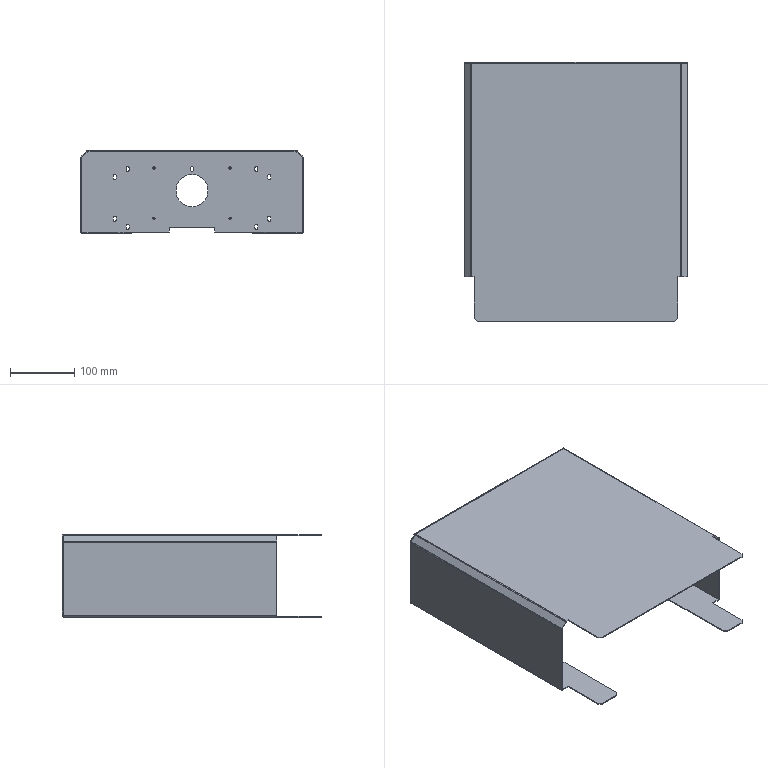Part | SolidWorks | features HoleWzd 3, ICE 3, Cut 2, FlatPattern 2, SheetMetal 2, SolidToSheetMetal 2, BreakCorner 1, Chamfer 1, EdgeFlange 1, Extrusion 1, MirrorPattern 1 | 2 solids | 145 faces | box 347 x 403 x 127.5 mm | volume 464397 mm3 | plane 86 | cylinder 59 | commonest cylinder face diameters 4.8 x27 3.3 x8 5.8 x8 1.473 x6 4.473 x6 50 x2